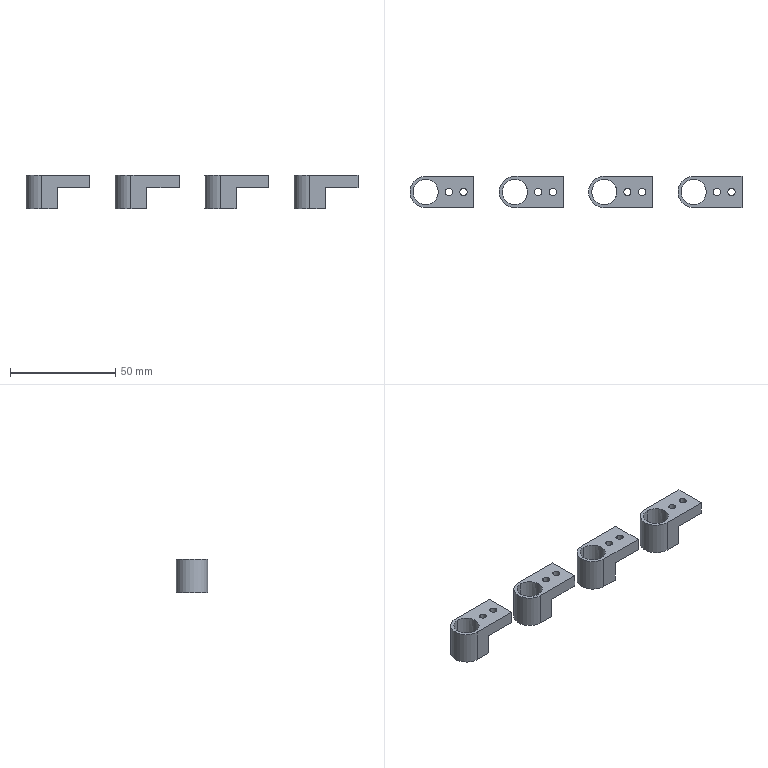NC program | NX | posted with a generic post | part box 158 x 15 x 16 mm
Lines 60 to 880 of 6389:
(ZLEVEL_PROFILE_1 , TOOL : D10)
N106 T04 M6
N108 G54
N110 G17 G0 G90 X-65.133 Y12.6 S7500 M3
N112 G43 Z30. H4
N114 Z1.5
N116 G94 G1 X-48.5 Z0.628 F1000.
N118 X-47.946 Z0.599
N120 X-46.602 Y12.266 Z0.527
N122 X-45.396 Y11.584 Z0.454
N124 X-44.416 Y10.604 Z0.381
N126 X-43.734 Y9.398 Z0.309
N128 X-43.4 Y8.054 Z0.236
N130 Y7.5 Z0.207
N132 Y-7.5 Z-0.579
N134 Y-8.054 Z-0.608
N136 X-43.734 Y-9.398 Z-0.681
N138 X-44.416 Y-10.604 Z-0.753
N140 X-45.396 Y-11.584 Z-0.826
N142 X-46.602 Y-12.266 Z-0.898
N144 X-47.946 Y-12.6 Z-0.971
N146 X-48.5 Z-1.
N148 X-71.5 F3000.
N150 G2 X-84.1 Y0. R12.6
N152 X-71.5 Y12.6 R12.6
N154 G1 X-48.5
N156 G2 X-43.4 Y7.5 R5.1
N158 G1 Y-7.5
N160 G2 X-48.5 Y-12.6 R5.1
N162 G1 X-70.951 Z-1.392
N164 X-71.339 Z-1.399
N166 X-71.726 Y-12.598 Z-1.405
N168 X-72.113 Y-12.585 Z-1.412
N170 X-72.499 Y-12.56 Z-1.419
N172 X-72.884 Y-12.524 Z-1.426
N174 X-73.268 Y-12.475 Z-1.432
N176 X-73.651 Y-12.415 Z-1.439
N178 X-74.031 Y-12.343 Z-1.446
N180 X-74.409 Y-12.26 Z-1.453
N182 X-74.784 Y-12.164 Z-1.459
N184 X-75.156 Y-12.058 Z-1.466
N186 X-75.525 Y-11.94 Z-1.473
N188 X-75.89 Y-11.811 Z-1.48
N190 X-76.25 Y-11.67 Z-1.486
N192 X-76.607 Y-11.519 Z-1.493
N194 X-76.958 Y-11.356 Z-1.5
N196 X-77.304 Y-11.183 Z-1.507
N198 X-77.645 Y-11. Z-1.514
N200 X-77.98 Y-10.806 Z-1.52
N202 X-78.309 Y-10.602 Z-1.527
N204 X-78.631 Y-10.388 Z-1.534
N206 X-78.947 Y-10.164 Z-1.541
N208 X-79.256 Y-9.93 Z-1.547
N210 X-79.557 Y-9.687 Z-1.554
N212 X-79.851 Y-9.435 Z-1.561
N214 X-80.137 Y-9.174 Z-1.568
N216 X-80.415 Y-8.905 Z-1.574
N218 X-80.684 Y-8.627 Z-1.581
N220 X-80.944 Y-8.34 Z-1.588
N222 X-81.196 Y-8.046 Z-1.595
N224 X-81.439 Y-7.745 Z-1.601
N226 X-81.672 Y-7.436 Z-1.608
N228 X-81.896 Y-7.12 Z-1.615
N230 X-82.109 Y-6.797 Z-1.622
N232 X-82.313 Y-6.468 Z-1.628
N234 X-82.507 Y-6.133 Z-1.635
N236 X-82.69 Y-5.792 Z-1.642
N238 X-82.863 Y-5.445 Z-1.649
N240 X-83.024 Y-5.094 Z-1.655
N242 X-83.175 Y-4.737 Z-1.662
N244 X-83.316 Y-4.377 Z-1.669
N246 X-83.444 Y-4.012 Z-1.676
N248 X-83.562 Y-3.643 Z-1.682
N250 X-83.668 Y-3.271 Z-1.689
N252 X-83.763 Y-2.895 Z-1.696
N254 X-83.846 Y-2.517 Z-1.703
N256 X-83.918 Y-2.137 Z-1.709
N258 X-83.977 Y-1.754 Z-1.716
N260 X-84.025 Y-1.37 Z-1.723
N262 X-84.061 Y-0.985 Z-1.73
N264 X-84.086 Y-0.599 Z-1.736
N266 X-84.098 Y-0.212 Z-1.743
N268 X-84.099 Y0.175 Z-1.75
N270 X-84.087 Y0.562 Z-1.757
N272 X-84.064 Y0.949 Z-1.764
N274 X-84.029 Y1.334 Z-1.77
N276 X-83.982 Y1.718 Z-1.777
N278 X-83.924 Y2.101 Z-1.784
N280 X-83.853 Y2.482 Z-1.791
N282 X-83.771 Y2.86 Z-1.797
N284 X-83.677 Y3.236 Z-1.804
N286 X-83.572 Y3.608 Z-1.811
N288 X-83.456 Y3.977 Z-1.818
N290 X-83.328 Y4.343 Z-1.824
N292 X-83.189 Y4.704 Z-1.831
N294 X-83.039 Y5.061 Z-1.838
N296 X-82.878 Y5.413 Z-1.845
N298 X-82.707 Y5.76 Z-1.851
N300 X-82.524 Y6.101 Z-1.858
N302 X-82.332 Y6.437 Z-1.865
N304 X-82.129 Y6.767 Z-1.872
N306 X-81.916 Y7.09 Z-1.878
N308 X-81.693 Y7.407 Z-1.885
N310 X-81.461 Y7.716 Z-1.892
N312 X-81.219 Y8.018 Z-1.899
N314 X-80.968 Y8.313 Z-1.905
N316 X-80.709 Y8.6 Z-1.912
N318 X-80.44 Y8.879 Z-1.919
N320 X-80.163 Y9.149 Z-1.926
N322 X-79.878 Y9.411 Z-1.932
N324 X-79.585 Y9.664 Z-1.939
N326 X-79.284 Y9.908 Z-1.946
N328 X-78.976 Y10.142 Z-1.953
N330 X-78.661 Y10.367 Z-1.959
N332 X-78.339 Y10.582 Z-1.966
N334 X-78.011 Y10.787 Z-1.973
N336 X-77.677 Y10.982 Z-1.98
N338 X-77.336 Y11.167 Z-1.986
N340 X-76.991 Y11.341 Z-1.993
N342 X-76.64 Y11.504 Z-2.
N344 G2 X-71.5 Y12.6 R12.6
N346 G1 X-48.5
N348 G2 X-43.4 Y7.5 R5.1
N350 G1 Y-7.5
N352 G2 X-48.5 Y-12.6 R5.1
N354 G1 X-70.951 Z-2.392
N356 X-71.339 Z-2.399
N358 X-71.726 Y-12.598 Z-2.405
N360 X-72.113 Y-12.585 Z-2.412
N362 X-72.499 Y-12.56 Z-2.419
N364 X-72.884 Y-12.524 Z-2.426
N366 X-73.268 Y-12.475 Z-2.432
N368 X-73.651 Y-12.415 Z-2.439
N370 X-74.031 Y-12.343 Z-2.446
N372 X-74.409 Y-12.26 Z-2.453
N374 X-74.784 Y-12.164 Z-2.459
N376 X-75.156 Y-12.058 Z-2.466
N378 X-75.525 Y-11.94 Z-2.473
N380 X-75.89 Y-11.811 Z-2.48
N382 X-76.25 Y-11.67 Z-2.486
N384 X-76.607 Y-11.519 Z-2.493
N386 X-76.958 Y-11.356 Z-2.5
N388 X-77.304 Y-11.183 Z-2.507
N390 X-77.645 Y-11. Z-2.514
N392 X-77.98 Y-10.806 Z-2.52
N394 X-78.309 Y-10.602 Z-2.527
N396 X-78.631 Y-10.388 Z-2.534
N398 X-78.947 Y-10.164 Z-2.541
N400 X-79.256 Y-9.93 Z-2.547
N402 X-79.557 Y-9.687 Z-2.554
N404 X-79.851 Y-9.435 Z-2.561
N406 X-80.137 Y-9.174 Z-2.568
N408 X-80.415 Y-8.905 Z-2.574
N410 X-80.684 Y-8.627 Z-2.581
N412 X-80.944 Y-8.34 Z-2.588
N414 X-81.196 Y-8.046 Z-2.595
N416 X-81.439 Y-7.745 Z-2.601
N418 X-81.672 Y-7.436 Z-2.608
N420 X-81.896 Y-7.12 Z-2.615
N422 X-82.109 Y-6.797 Z-2.622
N424 X-82.313 Y-6.468 Z-2.628
N426 X-82.507 Y-6.133 Z-2.635
N428 X-82.69 Y-5.792 Z-2.642
N430 X-82.863 Y-5.445 Z-2.649
N432 X-83.024 Y-5.094 Z-2.655
N434 X-83.175 Y-4.737 Z-2.662
N436 X-83.316 Y-4.377 Z-2.669
N438 X-83.444 Y-4.012 Z-2.676
N440 X-83.562 Y-3.643 Z-2.682
N442 X-83.668 Y-3.271 Z-2.689
N444 X-83.763 Y-2.895 Z-2.696
N446 X-83.846 Y-2.517 Z-2.703
N448 X-83.918 Y-2.137 Z-2.709
N450 X-83.977 Y-1.754 Z-2.716
N452 X-84.025 Y-1.37 Z-2.723
N454 X-84.061 Y-0.985 Z-2.73
N456 X-84.086 Y-0.599 Z-2.736
N458 X-84.098 Y-0.212 Z-2.743
N460 X-84.099 Y0.175 Z-2.75
N462 X-84.087 Y0.562 Z-2.757
N464 X-84.064 Y0.949 Z-2.764
N466 X-84.029 Y1.334 Z-2.77
N468 X-83.982 Y1.718 Z-2.777
N470 X-83.924 Y2.101 Z-2.784
N472 X-83.853 Y2.482 Z-2.791
N474 X-83.771 Y2.86 Z-2.797
N476 X-83.677 Y3.236 Z-2.804
N478 X-83.572 Y3.608 Z-2.811
N480 X-83.456 Y3.977 Z-2.818
N482 X-83.328 Y4.343 Z-2.824
N484 X-83.189 Y4.704 Z-2.831
N486 X-83.039 Y5.061 Z-2.838
N488 X-82.878 Y5.413 Z-2.845
N490 X-82.707 Y5.76 Z-2.851
N492 X-82.524 Y6.101 Z-2.858
N494 X-82.332 Y6.437 Z-2.865
N496 X-82.129 Y6.767 Z-2.872
N498 X-81.916 Y7.09 Z-2.878
N500 X-81.693 Y7.407 Z-2.885
N502 X-81.461 Y7.716 Z-2.892
N504 X-81.219 Y8.018 Z-2.899
N506 X-80.968 Y8.313 Z-2.905
N508 X-80.709 Y8.6 Z-2.912
N510 X-80.44 Y8.879 Z-2.919
N512 X-80.163 Y9.149 Z-2.926
N514 X-79.878 Y9.411 Z-2.932
N516 X-79.585 Y9.664 Z-2.939
N518 X-79.284 Y9.908 Z-2.946
N520 X-78.976 Y10.142 Z-2.953
N522 X-78.661 Y10.367 Z-2.959
N524 X-78.339 Y10.582 Z-2.966
N526 X-78.011 Y10.787 Z-2.973
N528 X-77.677 Y10.982 Z-2.98
N530 X-77.336 Y11.167 Z-2.986
N532 X-76.991 Y11.341 Z-2.993
N534 X-76.64 Y11.504 Z-3.
N536 G2 X-71.5 Y12.6 R12.6
N538 G1 X-48.5
N540 G2 X-43.4 Y7.5 R5.1
N542 G1 Y-7.5
N544 G2 X-48.5 Y-12.6 R5.1
N546 G1 X-70.951 Z-3.392
N548 X-71.339 Z-3.399
N550 X-71.726 Y-12.598 Z-3.405
N552 X-72.113 Y-12.585 Z-3.412
N554 X-72.499 Y-12.56 Z-3.419
N556 X-72.884 Y-12.524 Z-3.426
N558 X-73.268 Y-12.475 Z-3.432
N560 X-73.651 Y-12.415 Z-3.439
N562 X-74.031 Y-12.343 Z-3.446
N564 X-74.409 Y-12.26 Z-3.453
N566 X-74.784 Y-12.164 Z-3.459
N568 X-75.156 Y-12.058 Z-3.466
N570 X-75.525 Y-11.94 Z-3.473
N572 X-75.89 Y-11.811 Z-3.48
N574 X-76.25 Y-11.67 Z-3.486
N576 X-76.607 Y-11.519 Z-3.493
N578 X-76.958 Y-11.356 Z-3.5
N580 X-77.304 Y-11.183 Z-3.507
N582 X-77.645 Y-11. Z-3.514
N584 X-77.98 Y-10.806 Z-3.52
N586 X-78.309 Y-10.602 Z-3.527
N588 X-78.631 Y-10.388 Z-3.534
N590 X-78.947 Y-10.164 Z-3.541
N592 X-79.256 Y-9.93 Z-3.547
N594 X-79.557 Y-9.687 Z-3.554
N596 X-79.851 Y-9.435 Z-3.561
N598 X-80.137 Y-9.174 Z-3.568
N600 X-80.415 Y-8.905 Z-3.574
N602 X-80.684 Y-8.627 Z-3.581
N604 X-80.944 Y-8.34 Z-3.588
N606 X-81.196 Y-8.046 Z-3.595
N608 X-81.439 Y-7.745 Z-3.601
N610 X-81.672 Y-7.436 Z-3.608
N612 X-81.896 Y-7.12 Z-3.615
N614 X-82.109 Y-6.797 Z-3.622
N616 X-82.313 Y-6.468 Z-3.628
N618 X-82.507 Y-6.133 Z-3.635
N620 X-82.69 Y-5.792 Z-3.642
N622 X-82.863 Y-5.445 Z-3.649
N624 X-83.024 Y-5.094 Z-3.655
N626 X-83.175 Y-4.737 Z-3.662
N628 X-83.316 Y-4.377 Z-3.669
N630 X-83.444 Y-4.012 Z-3.676
N632 X-83.562 Y-3.643 Z-3.682
N634 X-83.668 Y-3.271 Z-3.689
N636 X-83.763 Y-2.895 Z-3.696
N638 X-83.846 Y-2.517 Z-3.703
N640 X-83.918 Y-2.137 Z-3.709
N642 X-83.977 Y-1.754 Z-3.716
N644 X-84.025 Y-1.37 Z-3.723
N646 X-84.061 Y-0.985 Z-3.73
N648 X-84.086 Y-0.599 Z-3.736
N650 X-84.098 Y-0.212 Z-3.743
N652 X-84.099 Y0.175 Z-3.75
N654 X-84.087 Y0.562 Z-3.757
N656 X-84.064 Y0.949 Z-3.764
N658 X-84.029 Y1.334 Z-3.77
N660 X-83.982 Y1.718 Z-3.777
N662 X-83.924 Y2.101 Z-3.784
N664 X-83.853 Y2.482 Z-3.791
N666 X-83.771 Y2.86 Z-3.797
N668 X-83.677 Y3.236 Z-3.804
N670 X-83.572 Y3.608 Z-3.811
N672 X-83.456 Y3.977 Z-3.818
N674 X-83.328 Y4.343 Z-3.824
N676 X-83.189 Y4.704 Z-3.831
N678 X-83.039 Y5.061 Z-3.838
N680 X-82.878 Y5.413 Z-3.845
N682 X-82.707 Y5.76 Z-3.851
N684 X-82.524 Y6.101 Z-3.858
N686 X-82.332 Y6.437 Z-3.865
N688 X-82.129 Y6.767 Z-3.872
N690 X-81.916 Y7.09 Z-3.878
N692 X-81.693 Y7.407 Z-3.885
N694 X-81.461 Y7.716 Z-3.892
N696 X-81.219 Y8.018 Z-3.899
N698 X-80.968 Y8.313 Z-3.905
N700 X-80.709 Y8.6 Z-3.912
N702 X-80.44 Y8.879 Z-3.919
N704 X-80.163 Y9.149 Z-3.926
N706 X-79.878 Y9.411 Z-3.932
N708 X-79.585 Y9.664 Z-3.939
N710 X-79.284 Y9.908 Z-3.946
N712 X-78.976 Y10.142 Z-3.953
N714 X-78.661 Y10.367 Z-3.959
N716 X-78.339 Y10.582 Z-3.966
N718 X-78.011 Y10.787 Z-3.973
N720 X-77.677 Y10.982 Z-3.98
N722 X-77.336 Y11.167 Z-3.986
N724 X-76.991 Y11.341 Z-3.993
N726 X-76.64 Y11.504 Z-4.
N728 G2 X-71.5 Y12.6 R12.6
N730 G1 X-48.5
N732 G2 X-43.4 Y7.5 R5.1
N734 G1 Y-7.5
N736 G2 X-48.5 Y-12.6 R5.1
N738 G1 X-70.951 Z-4.392
N740 X-71.339 Z-4.399
N742 X-71.726 Y-12.598 Z-4.405
N744 X-72.113 Y-12.585 Z-4.412
N746 X-72.499 Y-12.56 Z-4.419
N748 X-72.884 Y-12.524 Z-4.426
N750 X-73.268 Y-12.475 Z-4.432
N752 X-73.651 Y-12.415 Z-4.439
N754 X-74.031 Y-12.343 Z-4.446
N756 X-74.409 Y-12.26 Z-4.453
N758 X-74.784 Y-12.164 Z-4.459
N760 X-75.156 Y-12.058 Z-4.466
N762 X-75.525 Y-11.94 Z-4.473
N764 X-75.89 Y-11.811 Z-4.48
N766 X-76.25 Y-11.67 Z-4.486
N768 X-76.607 Y-11.519 Z-4.493
N770 X-76.958 Y-11.356 Z-4.5
N772 X-77.304 Y-11.183 Z-4.507
N774 X-77.645 Y-11. Z-4.514
N776 X-77.98 Y-10.806 Z-4.52
N778 X-78.309 Y-10.602 Z-4.527
N780 X-78.631 Y-10.388 Z-4.534
N782 X-78.947 Y-10.164 Z-4.541
N784 X-79.256 Y-9.93 Z-4.547
N786 X-79.557 Y-9.687 Z-4.554
N788 X-79.851 Y-9.435 Z-4.561
N790 X-80.137 Y-9.174 Z-4.568
N792 X-80.415 Y-8.905 Z-4.574
N794 X-80.684 Y-8.627 Z-4.581
N796 X-80.944 Y-8.34 Z-4.588
N798 X-81.196 Y-8.046 Z-4.595
N800 X-81.439 Y-7.745 Z-4.601
N802 X-81.672 Y-7.436 Z-4.608
N804 X-81.896 Y-7.12 Z-4.615
N806 X-82.109 Y-6.797 Z-4.622
N808 X-82.313 Y-6.468 Z-4.628
N810 X-82.507 Y-6.133 Z-4.635
N812 X-82.69 Y-5.792 Z-4.642
N814 X-82.863 Y-5.445 Z-4.649
N816 X-83.024 Y-5.094 Z-4.655
N818 X-83.175 Y-4.737 Z-4.662
N820 X-83.316 Y-4.377 Z-4.669
N822 X-83.444 Y-4.012 Z-4.676
N824 X-83.562 Y-3.643 Z-4.682
N826 X-83.668 Y-3.271 Z-4.689
N828 X-83.763 Y-2.895 Z-4.696
N830 X-83.846 Y-2.517 Z-4.703
N832 X-83.918 Y-2.137 Z-4.709
N834 X-83.977 Y-1.754 Z-4.716
N836 X-84.025 Y-1.37 Z-4.723
N838 X-84.061 Y-0.985 Z-4.73
N840 X-84.086 Y-0.599 Z-4.736
N842 X-84.098 Y-0.212 Z-4.743
N844 X-84.099 Y0.175 Z-4.75
N846 X-84.087 Y0.562 Z-4.757
N848 X-84.064 Y0.949 Z-4.764
N850 X-84.029 Y1.334 Z-4.77
N852 X-83.982 Y1.718 Z-4.777
N854 X-83.924 Y2.101 Z-4.784
N856 X-83.853 Y2.482 Z-4.791
N858 X-83.771 Y2.86 Z-4.797
N860 X-83.677 Y3.236 Z-4.804
N862 X-83.572 Y3.608 Z-4.811
N864 X-83.456 Y3.977 Z-4.818
N866 X-83.328 Y4.343 Z-4.824
N868 X-83.189 Y4.704 Z-4.831
N870 X-83.039 Y5.061 Z-4.838
N872 X-82.878 Y5.413 Z-4.845
N874 X-82.707 Y5.76 Z-4.851
N876 X-82.524 Y6.101 Z-4.858
N878 X-82.332 Y6.437 Z-4.865
N880 X-82.129 Y6.767 Z-4.872
N882 X-81.916 Y7.09 Z-4.878
N884 X-81.693 Y7.407 Z-4.885
N886 X-81.461 Y7.716 Z-4.892
N888 X-81.219 Y8.018 Z-4.899
N890 X-80.968 Y8.313 Z-4.905
N892 X-80.709 Y8.6 Z-4.912
N894 X-80.44 Y8.879 Z-4.919
N896 X-80.163 Y9.149 Z-4.926
N898 X-79.878 Y9.411 Z-4.932
N900 X-79.585 Y9.664 Z-4.939
N902 X-79.284 Y9.908 Z-4.946
N904 X-78.976 Y10.142 Z-4.953
N906 X-78.661 Y10.367 Z-4.959
N908 X-78.339 Y10.582 Z-4.966
N910 X-78.011 Y10.787 Z-4.973
N912 X-77.677 Y10.982 Z-4.98
N914 X-77.336 Y11.167 Z-4.986
N916 X-76.991 Y11.341 Z-4.993
N918 X-76.64 Y11.504 Z-5.
N920 G2 X-71.5 Y12.6 R12.6
N922 G1 X-48.5
N924 G2 X-43.4 Y7.5 R5.1
N926 G1 Y-7.5
N928 G2 X-48.5 Y-12.6 R5.1
N930 G1 X-70.951 Z-5.392
N932 X-71.339 Z-5.399
N934 X-71.726 Y-12.598 Z-5.405
N936 X-72.113 Y-12.585 Z-5.412
N938 X-72.499 Y-12.56 Z-5.419
N940 X-72.884 Y-12.524 Z-5.426
N942 X-73.268 Y-12.475 Z-5.432
N944 X-73.651 Y-12.415 Z-5.439
N946 X-74.031 Y-12.343 Z-5.446
N948 X-74.409 Y-12.26 Z-5.453
N950 X-74.784 Y-12.164 Z-5.459
N952 X-75.156 Y-12.058 Z-5.466
N954 X-75.525 Y-11.94 Z-5.473
N956 X-75.89 Y-11.811 Z-5.48
N958 X-76.25 Y-11.67 Z-5.486
N960 X-76.607 Y-11.519 Z-5.493
N962 X-76.958 Y-11.356 Z-5.5
N964 X-77.304 Y-11.183 Z-5.507
N966 X-77.645 Y-11. Z-5.514
N968 X-77.98 Y-10.806 Z-5.52
N970 X-78.309 Y-10.602 Z-5.527
N972 X-78.631 Y-10.388 Z-5.534
N974 X-78.947 Y-10.164 Z-5.541
N976 X-79.256 Y-9.93 Z-5.547
N978 X-79.557 Y-9.687 Z-5.554
N980 X-79.851 Y-9.435 Z-5.561
N982 X-80.137 Y-9.174 Z-5.568
N984 X-80.415 Y-8.905 Z-5.574
N986 X-80.684 Y-8.627 Z-5.581
N988 X-80.944 Y-8.34 Z-5.588
N990 X-81.196 Y-8.046 Z-5.595
N992 X-81.439 Y-7.745 Z-5.601
N994 X-81.672 Y-7.436 Z-5.608
N996 X-81.896 Y-7.12 Z-5.615
N998 X-82.109 Y-6.797 Z-5.622
N1000 X-82.313 Y-6.468 Z-5.628
N1002 X-82.507 Y-6.133 Z-5.635
N1004 X-82.69 Y-5.792 Z-5.642
N1006 X-82.863 Y-5.445 Z-5.649
N1008 X-83.024 Y-5.094 Z-5.655
N1010 X-83.175 Y-4.737 Z-5.662
N1012 X-83.316 Y-4.377 Z-5.669
N1014 X-83.444 Y-4.012 Z-5.676
N1016 X-83.562 Y-3.643 Z-5.682
N1018 X-83.668 Y-3.271 Z-5.689
N1020 X-83.763 Y-2.895 Z-5.696
N1022 X-83.846 Y-2.517 Z-5.703
N1024 X-83.918 Y-2.137 Z-5.709
N1026 X-83.977 Y-1.754 Z-5.716
N1028 X-84.025 Y-1.37 Z-5.723
N1030 X-84.061 Y-0.985 Z-5.73
N1032 X-84.086 Y-0.599 Z-5.736
N1034 X-84.098 Y-0.212 Z-5.743
N1036 X-84.099 Y0.175 Z-5.75
N1038 X-84.087 Y0.562 Z-5.757
N1040 X-84.064 Y0.949 Z-5.764
N1042 X-84.029 Y1.334 Z-5.77
N1044 X-83.982 Y1.718 Z-5.777
N1046 X-83.924 Y2.101 Z-5.784
N1048 X-83.853 Y2.482 Z-5.791
N1050 X-83.771 Y2.86 Z-5.797
N1052 X-83.677 Y3.236 Z-5.804
N1054 X-83.572 Y3.608 Z-5.811
N1056 X-83.456 Y3.977 Z-5.818
N1058 X-83.328 Y4.343 Z-5.824
N1060 X-83.189 Y4.704 Z-5.831
N1062 X-83.039 Y5.061 Z-5.838
N1064 X-82.878 Y5.413 Z-5.845
N1066 X-82.707 Y5.76 Z-5.851
N1068 X-82.524 Y6.101 Z-5.858
N1070 X-82.332 Y6.437 Z-5.865
N1072 X-82.129 Y6.767 Z-5.872
N1074 X-81.916 Y7.09 Z-5.878
N1076 X-81.693 Y7.407 Z-5.885
N1078 X-81.461 Y7.716 Z-5.892
N1080 X-81.219 Y8.018 Z-5.899
N1082 X-80.968 Y8.313 Z-5.905
N1084 X-80.709 Y8.6 Z-5.912
N1086 X-80.44 Y8.879 Z-5.919
N1088 X-80.163 Y9.149 Z-5.926
N1090 X-79.878 Y9.411 Z-5.932
N1092 X-79.585 Y9.664 Z-5.939
N1094 X-79.284 Y9.908 Z-5.946
N1096 X-78.976 Y10.142 Z-5.953
N1098 X-78.661 Y10.367 Z-5.959
N1100 X-78.339 Y10.582 Z-5.966
N1102 X-78.011 Y10.787 Z-5.973
N1104 X-77.677 Y10.982 Z-5.98
N1106 X-77.336 Y11.167 Z-5.986
N1108 X-76.991 Y11.341 Z-5.993
N1110 X-76.64 Y11.504 Z-6.
N1112 G2 X-71.5 Y12.6 R12.6
N1114 G1 X-48.5
N1116 G2 X-43.4 Y7.5 R5.1
N1118 G1 Y-7.5
N1120 G2 X-48.5 Y-12.6 R5.1
N1122 G1 X-70.951 Z-6.392
N1124 X-71.339 Z-6.399
N1126 X-71.726 Y-12.598 Z-6.405
N1128 X-72.113 Y-12.585 Z-6.412
N1130 X-72.499 Y-12.56 Z-6.419
N1132 X-72.884 Y-12.524 Z-6.426
N1134 X-73.268 Y-12.475 Z-6.432
N1136 X-73.651 Y-12.415 Z-6.439
N1138 X-74.031 Y-12.343 Z-6.446
N1140 X-74.409 Y-12.26 Z-6.453
N1142 X-74.784 Y-12.164 Z-6.459
N1144 X-75.156 Y-12.058 Z-6.466
N1146 X-75.525 Y-11.94 Z-6.473
N1148 X-75.89 Y-11.811 Z-6.48
N1150 X-76.25 Y-11.67 Z-6.486
N1152 X-76.607 Y-11.519 Z-6.493
N1154 X-76.958 Y-11.356 Z-6.5
N1156 X-77.304 Y-11.183 Z-6.507
N1158 X-77.645 Y-11. Z-6.514
N1160 X-77.98 Y-10.806 Z-6.52
N1162 X-78.309 Y-10.602 Z-6.527
N1164 X-78.631 Y-10.388 Z-6.534
N1166 X-78.947 Y-10.164 Z-6.541
N1168 X-79.256 Y-9.93 Z-6.547
N1170 X-79.557 Y-9.687 Z-6.554
N1172 X-79.851 Y-9.435 Z-6.561
N1174 X-80.137 Y-9.174 Z-6.568
N1176 X-80.415 Y-8.905 Z-6.574
N1178 X-80.684 Y-8.627 Z-6.581
N1180 X-80.944 Y-8.34 Z-6.588
N1182 X-81.196 Y-8.046 Z-6.595
N1184 X-81.439 Y-7.745 Z-6.601
N1186 X-81.672 Y-7.436 Z-6.608
N1188 X-81.896 Y-7.12 Z-6.615
N1190 X-82.109 Y-6.797 Z-6.622
N1192 X-82.313 Y-6.468 Z-6.628
N1194 X-82.507 Y-6.133 Z-6.635
N1196 X-82.69 Y-5.792 Z-6.642
N1198 X-82.863 Y-5.445 Z-6.649
N1200 X-83.024 Y-5.094 Z-6.655
N1202 X-83.175 Y-4.737 Z-6.662
N1204 X-83.316 Y-4.377 Z-6.669
N1206 X-83.444 Y-4.012 Z-6.676
N1208 X-83.562 Y-3.643 Z-6.682
N1210 X-83.668 Y-3.271 Z-6.689
N1212 X-83.763 Y-2.895 Z-6.696
N1214 X-83.846 Y-2.517 Z-6.703
N1216 X-83.918 Y-2.137 Z-6.709
N1218 X-83.977 Y-1.754 Z-6.716
N1220 X-84.025 Y-1.37 Z-6.723
N1222 X-84.061 Y-0.985 Z-6.73
N1224 X-84.086 Y-0.599 Z-6.736
N1226 X-84.098 Y-0.212 Z-6.743
N1228 X-84.099 Y0.175 Z-6.75
N1230 X-84.087 Y0.562 Z-6.757
N1232 X-84.064 Y0.949 Z-6.764
N1234 X-84.029 Y1.334 Z-6.77
N1236 X-83.982 Y1.718 Z-6.777
N1238 X-83.924 Y2.101 Z-6.784
N1240 X-83.853 Y2.482 Z-6.791
N1242 X-83.771 Y2.86 Z-6.797
N1244 X-83.677 Y3.236 Z-6.804
N1246 X-83.572 Y3.608 Z-6.811
N1248 X-83.456 Y3.977 Z-6.818
N1250 X-83.328 Y4.343 Z-6.824
N1252 X-83.189 Y4.704 Z-6.831
N1254 X-83.039 Y5.061 Z-6.838
N1256 X-82.878 Y5.413 Z-6.845
N1258 X-82.707 Y5.76 Z-6.851
N1260 X-82.524 Y6.101 Z-6.858
N1262 X-82.332 Y6.437 Z-6.865
N1264 X-82.129 Y6.767 Z-6.872
N1266 X-81.916 Y7.09 Z-6.878
N1268 X-81.693 Y7.407 Z-6.885
N1270 X-81.461 Y7.716 Z-6.892
N1272 X-81.219 Y8.018 Z-6.899
N1274 X-80.968 Y8.313 Z-6.905
N1276 X-80.709 Y8.6 Z-6.912
N1278 X-80.44 Y8.879 Z-6.919
N1280 X-80.163 Y9.149 Z-6.926
N1282 X-79.878 Y9.411 Z-6.932
N1284 X-79.585 Y9.664 Z-6.939
N1286 X-79.284 Y9.908 Z-6.946
N1288 X-78.976 Y10.142 Z-6.953
N1290 X-78.661 Y10.367 Z-6.959
N1292 X-78.339 Y10.582 Z-6.966
N1294 X-78.011 Y10.787 Z-6.973
N1296 X-77.677 Y10.982 Z-6.98
N1298 X-77.336 Y11.167 Z-6.986
N1300 X-76.991 Y11.341 Z-6.993
N1302 X-76.64 Y11.504 Z-7.
N1304 G2 X-71.5 Y12.6 R12.6
N1306 G1 X-48.5
N1308 G2 X-43.4 Y7.5 R5.1
N1310 G1 Y-7.5
N1312 G2 X-48.5 Y-12.6 R5.1
N1314 G1 X-70.951 Z-7.392
N1316 X-71.339 Z-7.399
N1318 X-71.726 Y-12.598 Z-7.405
N1320 X-72.113 Y-12.585 Z-7.412
N1322 X-72.499 Y-12.56 Z-7.419
N1324 X-72.884 Y-12.524 Z-7.426
N1326 X-73.268 Y-12.475 Z-7.432
N1328 X-73.651 Y-12.415 Z-7.439
N1330 X-74.031 Y-12.343 Z-7.446
N1332 X-74.409 Y-12.26 Z-7.453
N1334 X-74.784 Y-12.164 Z-7.459
N1336 X-75.156 Y-12.058 Z-7.466
N1338 X-75.525 Y-11.94 Z-7.473
N1340 X-75.89 Y-11.811 Z-7.48
N1342 X-76.25 Y-11.67 Z-7.486
N1344 X-76.607 Y-11.519 Z-7.493
N1346 X-76.958 Y-11.356 Z-7.5
N1348 X-77.304 Y-11.183 Z-7.507
N1350 X-77.645 Y-11. Z-7.514
N1352 X-77.98 Y-10.806 Z-7.52
N1354 X-78.309 Y-10.602 Z-7.527
N1356 X-78.631 Y-10.388 Z-7.534
N1358 X-78.947 Y-10.164 Z-7.541
N1360 X-79.256 Y-9.93 Z-7.547
N1362 X-79.557 Y-9.687 Z-7.554
N1364 X-79.851 Y-9.435 Z-7.561
N1366 X-80.137 Y-9.174 Z-7.568
N1368 X-80.415 Y-8.905 Z-7.574
N1370 X-80.684 Y-8.627 Z-7.581
N1372 X-80.944 Y-8.34 Z-7.588
N1374 X-81.196 Y-8.046 Z-7.595
N1376 X-81.439 Y-7.745 Z-7.601
N1378 X-81.672 Y-7.436 Z-7.608
N1380 X-81.896 Y-7.12 Z-7.615
N1382 X-82.109 Y-6.797 Z-7.622
N1384 X-82.313 Y-6.468 Z-7.628
N1386 X-82.507 Y-6.133 Z-7.635
N1388 X-82.69 Y-5.792 Z-7.642
N1390 X-82.863 Y-5.445 Z-7.649
N1392 X-83.024 Y-5.094 Z-7.655
N1394 X-83.175 Y-4.737 Z-7.662
N1396 X-83.316 Y-4.377 Z-7.669
N1398 X-83.444 Y-4.012 Z-7.676
N1400 X-83.562 Y-3.643 Z-7.682
N1402 X-83.668 Y-3.271 Z-7.689
N1404 X-83.763 Y-2.895 Z-7.696
N1406 X-83.846 Y-2.517 Z-7.703
N1408 X-83.918 Y-2.137 Z-7.709
N1410 X-83.977 Y-1.754 Z-7.716
N1412 X-84.025 Y-1.37 Z-7.723
N1414 X-84.061 Y-0.985 Z-7.73
N1416 X-84.086 Y-0.599 Z-7.736
N1418 X-84.098 Y-0.212 Z-7.743
N1420 X-84.099 Y0.175 Z-7.75
N1422 X-84.087 Y0.562 Z-7.757
N1424 X-84.064 Y0.949 Z-7.764
N1426 X-84.029 Y1.334 Z-7.77
N1428 X-83.982 Y1.718 Z-7.777
N1430 X-83.924 Y2.101 Z-7.784
N1432 X-83.853 Y2.482 Z-7.791
N1434 X-83.771 Y2.86 Z-7.797
N1436 X-83.677 Y3.236 Z-7.804
N1438 X-83.572 Y3.608 Z-7.811
N1440 X-83.456 Y3.977 Z-7.818
N1442 X-83.328 Y4.343 Z-7.824
N1444 X-83.189 Y4.704 Z-7.831
N1446 X-83.039 Y5.061 Z-7.838
N1448 X-82.878 Y5.413 Z-7.845
N1450 X-82.707 Y5.76 Z-7.851
N1452 X-82.524 Y6.101 Z-7.858
N1454 X-82.332 Y6.437 Z-7.865
N1456 X-82.129 Y6.767 Z-7.872
N1458 X-81.916 Y7.09 Z-7.878
N1460 X-81.693 Y7.407 Z-7.885
N1462 X-81.461 Y7.716 Z-7.892
N1464 X-81.219 Y8.018 Z-7.899
N1466 X-80.968 Y8.313 Z-7.905
N1468 X-80.709 Y8.6 Z-7.912
N1470 X-80.44 Y8.879 Z-7.919
N1472 X-80.163 Y9.149 Z-7.926
N1474 X-79.878 Y9.411 Z-7.932
N1476 X-79.585 Y9.664 Z-7.939
N1478 X-79.284 Y9.908 Z-7.946
N1480 X-78.976 Y10.142 Z-7.953
N1482 X-78.661 Y10.367 Z-7.959
N1484 X-78.339 Y10.582 Z-7.966
N1486 X-78.011 Y10.787 Z-7.973
N1488 X-77.677 Y10.982 Z-7.98
N1490 X-77.336 Y11.167 Z-7.986
N1492 X-76.991 Y11.341 Z-7.993
N1494 X-76.64 Y11.504 Z-8.
N1496 G2 X-71.5 Y12.6 R12.6
N1498 G1 X-48.5
N1500 G2 X-43.4 Y7.5 R5.1
N1502 G1 Y-7.5
N1504 G2 X-48.5 Y-12.6 R5.1
N1506 G1 X-70.951 Z-8.392
N1508 X-71.339 Z-8.399
N1510 X-71.726 Y-12.598 Z-8.405
N1512 X-72.113 Y-12.585 Z-8.412
N1514 X-72.499 Y-12.56 Z-8.419
N1516 X-72.884 Y-12.524 Z-8.426
N1518 X-73.268 Y-12.475 Z-8.432
N1520 X-73.651 Y-12.415 Z-8.439
N1522 X-74.031 Y-12.343 Z-8.446
N1524 X-74.409 Y-12.26 Z-8.453
N1526 X-74.784 Y-12.164 Z-8.459
N1528 X-75.156 Y-12.058 Z-8.466
N1530 X-75.525 Y-11.94 Z-8.473
N1532 X-75.89 Y-11.811 Z-8.48
N1534 X-76.25 Y-11.67 Z-8.486
N1536 X-76.607 Y-11.519 Z-8.493
N1538 X-76.958 Y-11.356 Z-8.5
N1540 X-77.304 Y-11.183 Z-8.507
N1542 X-77.645 Y-11. Z-8.514
N1544 X-77.98 Y-10.806 Z-8.52
N1546 X-78.309 Y-10.602 Z-8.527
N1548 X-78.631 Y-10.388 Z-8.534
N1550 X-78.947 Y-10.164 Z-8.541
N1552 X-79.256 Y-9.93 Z-8.547
N1554 X-79.557 Y-9.687 Z-8.554
N1556 X-79.851 Y-9.435 Z-8.561
N1558 X-80.137 Y-9.174 Z-8.568
N1560 X-80.415 Y-8.905 Z-8.574
N1562 X-80.684 Y-8.627 Z-8.581
N1564 X-80.944 Y-8.34 Z-8.588
N1566 X-81.196 Y-8.046 Z-8.595
N1568 X-81.439 Y-7.745 Z-8.601
N1570 X-81.672 Y-7.436 Z-8.608
N1572 X-81.896 Y-7.12 Z-8.615
N1574 X-82.109 Y-6.797 Z-8.622
N1576 X-82.313 Y-6.468 Z-8.628
N1578 X-82.507 Y-6.133 Z-8.635
N1580 X-82.69 Y-5.792 Z-8.642
N1582 X-82.863 Y-5.445 Z-8.649
N1584 X-83.024 Y-5.094 Z-8.655
N1586 X-83.175 Y-4.737 Z-8.662
N1588 X-83.316 Y-4.377 Z-8.669
N1590 X-83.444 Y-4.012 Z-8.676
N1592 X-83.562 Y-3.643 Z-8.682
N1594 X-83.668 Y-3.271 Z-8.689
N1596 X-83.763 Y-2.895 Z-8.696
N1598 X-83.846 Y-2.517 Z-8.703
N1600 X-83.918 Y-2.137 Z-8.709
N1602 X-83.977 Y-1.754 Z-8.716
N1604 X-84.025 Y-1.37 Z-8.723
N1606 X-84.061 Y-0.985 Z-8.73
N1608 X-84.086 Y-0.599 Z-8.736
N1610 X-84.098 Y-0.212 Z-8.743
N1612 X-84.099 Y0.175 Z-8.75
N1614 X-84.087 Y0.562 Z-8.757
N1616 X-84.064 Y0.949 Z-8.764
N1618 X-84.029 Y1.334 Z-8.77
N1620 X-83.982 Y1.718 Z-8.777
N1622 X-83.924 Y2.101 Z-8.784
N1624 X-83.853 Y2.482 Z-8.791
N1626 X-83.771 Y2.86 Z-8.797
N1628 X-83.677 Y3.236 Z-8.804
N1630 X-83.572 Y3.608 Z-8.811
N1632 X-83.456 Y3.977 Z-8.818
N1634 X-83.328 Y4.343 Z-8.824
N1636 X-83.189 Y4.704 Z-8.831
N1638 X-83.039 Y5.061 Z-8.838
N1640 X-82.878 Y5.413 Z-8.845
N1642 X-82.707 Y5.76 Z-8.851
N1644 X-82.524 Y6.101 Z-8.858
N1646 X-82.332 Y6.437 Z-8.865
N1648 X-82.129 Y6.767 Z-8.872
N1650 X-81.916 Y7.09 Z-8.878
N1652 X-81.693 Y7.407 Z-8.885
N1654 X-81.461 Y7.716 Z-8.892
N1656 X-81.219 Y8.018 Z-8.899
N1658 X-80.968 Y8.313 Z-8.905
N1660 X-80.709 Y8.6 Z-8.912
N1662 X-80.44 Y8.879 Z-8.919
N1664 X-80.163 Y9.149 Z-8.926
N1666 X-79.878 Y9.411 Z-8.932
N1668 X-79.585 Y9.664 Z-8.939
N1670 X-79.284 Y9.908 Z-8.946
N1672 X-78.976 Y10.142 Z-8.953
N1674 X-78.661 Y10.367 Z-8.959
N1676 X-78.339 Y10.582 Z-8.966
N1678 X-78.011 Y10.787 Z-8.973
N1680 X-77.677 Y10.982 Z-8.98
N1682 X-77.336 Y11.167 Z-8.986
N1684 X-76.991 Y11.341 Z-8.993
N1686 X-76.64 Y11.504 Z-9.
N1688 G2 X-71.5 Y12.6 R12.6
N1690 G1 X-48.5
N1692 G2 X-43.4 Y7.5 R5.1
N1694 G1 Y-7.5
N1696 G2 X-48.5 Y-12.6 R5.1
N1698 G1 X-70.951 Z-9.392
N1700 X-71.339 Z-9.399
N1702 X-71.726 Y-12.598 Z-9.405
N1704 X-72.113 Y-12.585 Z-9.412
N1706 X-72.499 Y-12.56 Z-9.419
N1708 X-72.884 Y-12.524 Z-9.426
N1710 X-73.268 Y-12.475 Z-9.432
N1712 X-73.651 Y-12.415 Z-9.439
N1714 X-74.031 Y-12.343 Z-9.446
N1716 X-74.409 Y-12.26 Z-9.453
N1718 X-74.784 Y-12.164 Z-9.459
N1720 X-75.156 Y-12.058 Z-9.466
N1722 X-75.525 Y-11.94 Z-9.473
N1724 X-75.89 Y-11.811 Z-9.48
N1726 X-76.25 Y-11.67 Z-9.486
N1728 X-76.607 Y-11.519 Z-9.493
N1730 X-76.958 Y-11.356 Z-9.5
N1732 X-77.304 Y-11.183 Z-9.507
N1734 X-77.645 Y-11. Z-9.514
N1736 X-77.98 Y-10.806 Z-9.52
N1738 X-78.309 Y-10.602 Z-9.527
N1740 X-78.631 Y-10.388 Z-9.534